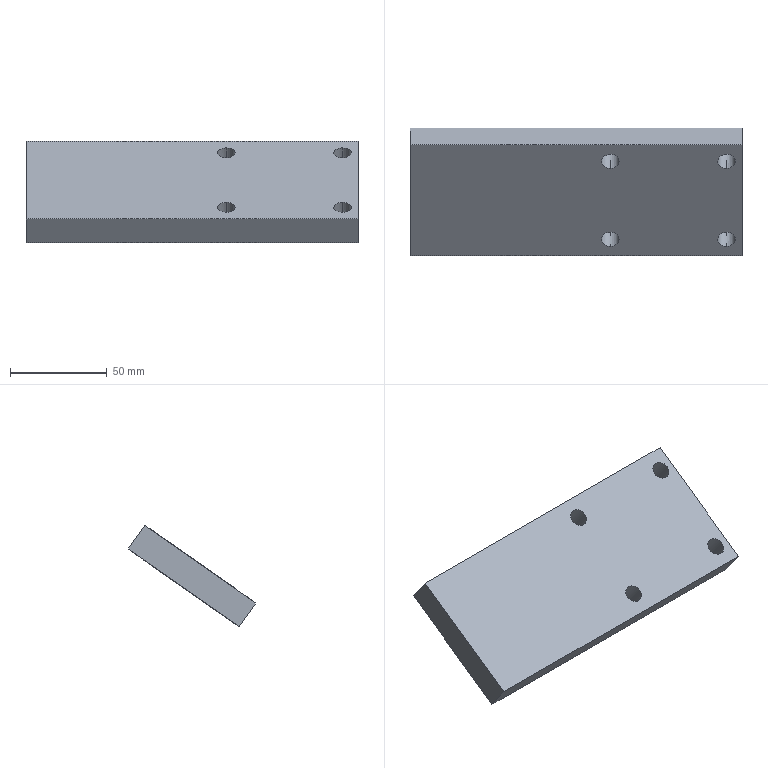Part | STEP file | Positioning_id1738_x_t | 1 solid | 14 faces | box 171.5 x 65.944 x 52.438 mm | volume 176258 mm3 | cylinder 8 | plane 6 | commonest cylinder face diameters 9 x8